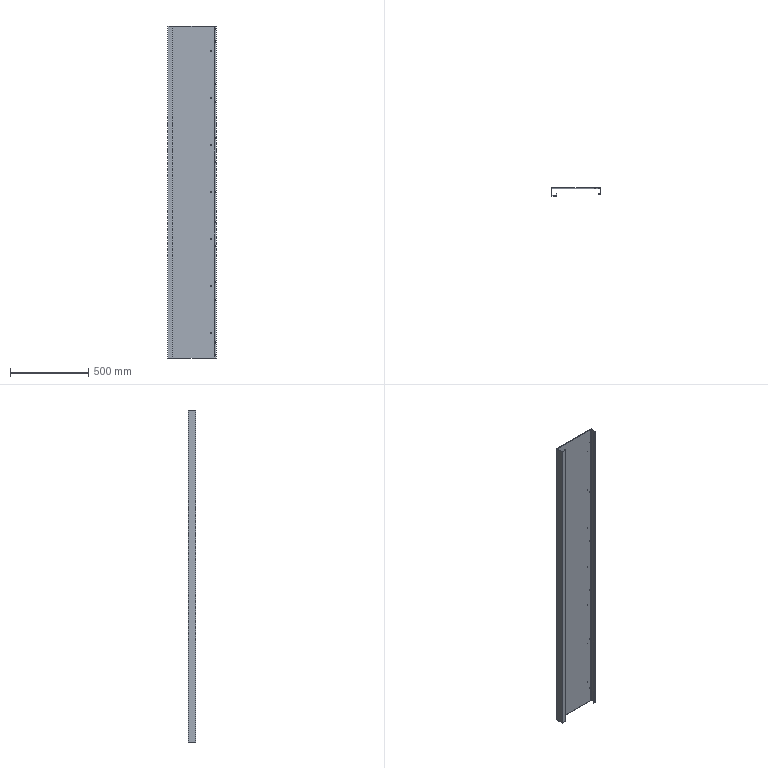Part | SolidWorks | features ICE 7, EdgeFlange 2, Cut 1, FlatPattern 1, SMBaseFlange 1, SheetMetal 1 | 1 solid | 130 faces | box 310.5 x 50 x 2116 mm | volume 1139747 mm3 | cylinder 76 | plane 54 | commonest cylinder face diameters 6.2 x28 4.2 x14 8 x12 11 x12 1 x5 3.4 x5